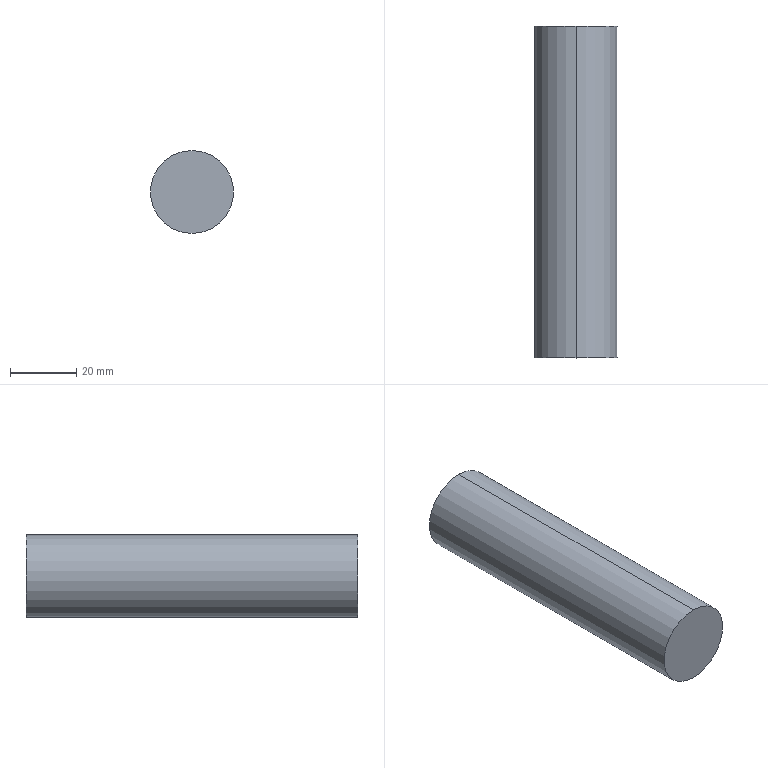Part | SolidWorks | features Extrusion 1 | 1 solid | 4 faces | box 25 x 100 x 25 mm | volume 49087 mm3 | cylinder 2 | plane 2 | commonest cylinder face diameters 25 x2
STEP:
#1=CARTESIAN_POINT('',(0.,100.,12.5));
#2=VERTEX_POINT('',#1);
#3=CARTESIAN_POINT('',(0.,100.,-12.5));
#4=VERTEX_POINT('',#3);
#5=CARTESIAN_POINT('',(0.,100.,0.));
#6=DIRECTION('',(0.,1.,0.));
#7=DIRECTION('',(0.,0.,1.));
#8=AXIS2_PLACEMENT_3D('',#5,#6,#7);
#9=CIRCLE('',#8,12.5);
#10=EDGE_CURVE('',#2,#4,#9,.T.);
#11=ORIENTED_EDGE('',*,*,#10,.F.);
#12=CARTESIAN_POINT('',(0.,0.,12.5));
#13=VERTEX_POINT('',#12);
#14=CARTESIAN_POINT('',(0.,100.,12.5));
#15=DIRECTION('',(0.,-1.,0.));
#16=VECTOR('',#15,1000.);
#17=LINE('',#14,#16);
#18=EDGE_CURVE('',#2,#13,#17,.T.);
#19=ORIENTED_EDGE('',*,*,#18,.T.);
#20=CARTESIAN_POINT('',(0.,0.,-12.5));
#21=VERTEX_POINT('',#20);
#22=CARTESIAN_POINT('',(0.,0.,0.));
#23=DIRECTION('',(0.,1.,0.));
#24=DIRECTION('',(0.,0.,1.));
#25=AXIS2_PLACEMENT_3D('',#22,#23,#24);
#26=CIRCLE('',#25,12.5);
#27=EDGE_CURVE('',#13,#21,#26,.T.);
#28=ORIENTED_EDGE('',*,*,#27,.T.);
#29=CARTESIAN_POINT('',(0.,100.,-12.5));
#30=DIRECTION('',(0.,-1.,0.));
#31=VECTOR('',#30,1000.);
#32=LINE('',#29,#31);
#33=EDGE_CURVE('',#4,#21,#32,.T.);
#34=ORIENTED_EDGE('',*,*,#33,.F.);
#35=EDGE_LOOP('',(#11,#19,#28,#34));
#36=FACE_OUTER_BOUND('',#35,.T.);
#37=CARTESIAN_POINT('',(0.,100.,0.));
#38=DIRECTION('',(0.,-1.,0.));
#39=DIRECTION('',(0.,0.,-1.));
#40=AXIS2_PLACEMENT_3D('',#37,#38,#39);
#41=CYLINDRICAL_SURFACE('',#40,12.5);
#42=ADVANCED_FACE('',(#36),#41,.T.);
#43=ORIENTED_EDGE('',*,*,#18,.F.);
#44=CARTESIAN_POINT('',(0.,100.,0.));
#45=DIRECTION('',(0.,1.,0.));
#46=DIRECTION('',(0.,0.,1.));
#47=AXIS2_PLACEMENT_3D('',#44,#45,#46);
#48=CIRCLE('',#47,12.5);
#49=EDGE_CURVE('',#4,#2,#48,.T.);
#50=ORIENTED_EDGE('',*,*,#49,.F.);
#51=ORIENTED_EDGE('',*,*,#33,.T.);
#52=CARTESIAN_POINT('',(0.,0.,0.));
#53=DIRECTION('',(0.,1.,0.));
#54=DIRECTION('',(0.,0.,1.));
#55=AXIS2_PLACEMENT_3D('',#52,#53,#54);
#56=CIRCLE('',#55,12.5);
#57=EDGE_CURVE('',#21,#13,#56,.T.);
#58=ORIENTED_EDGE('',*,*,#57,.T.);
#59=EDGE_LOOP('',(#43,#50,#51,#58));
#60=FACE_OUTER_BOUND('',#59,.T.);
#61=CARTESIAN_POINT('',(0.,100.,0.));
#62=DIRECTION('',(0.,-1.,0.));
#63=DIRECTION('',(0.,0.,-1.));
#64=AXIS2_PLACEMENT_3D('',#61,#62,#63);
#65=CYLINDRICAL_SURFACE('',#64,12.5);
#66=ADVANCED_FACE('',(#60),#65,.T.);
#67=ORIENTED_EDGE('',*,*,#49,.T.);
#68=ORIENTED_EDGE('',*,*,#10,.T.);
#69=EDGE_LOOP('',(#67,#68));
#70=FACE_OUTER_BOUND('',#69,.T.);
#71=CARTESIAN_POINT('',(0.,100.,0.));
#72=DIRECTION('',(0.,1.,0.));
#73=DIRECTION('',(0.,0.,1.));
#74=AXIS2_PLACEMENT_3D('',#71,#72,#73);
#75=PLANE('',#74);
#76=ADVANCED_FACE('',(#70),#75,.T.);
#77=ORIENTED_EDGE('',*,*,#57,.F.);
#78=ORIENTED_EDGE('',*,*,#27,.F.);
#79=EDGE_LOOP('',(#77,#78));
#80=FACE_OUTER_BOUND('',#79,.T.);
#81=CARTESIAN_POINT('',(0.,0.,0.));
#82=DIRECTION('',(0.,1.,0.));
#83=DIRECTION('',(0.,0.,1.));
#84=AXIS2_PLACEMENT_3D('',#81,#82,#83);
#85=PLANE('',#84);
#86=ADVANCED_FACE('',(#80),#85,.F.);
#87=CLOSED_SHELL('',(#42,#66,#76,#86));
#88=MANIFOLD_SOLID_BREP('',#87);
#89=CARTESIAN_POINT('',(0.,0.,0.));
#90=DIRECTION('',(0.,0.,1.));
#91=DIRECTION('',(1.,0.,0.));
#92=AXIS2_PLACEMENT_3D('',#89,#90,#91);
#93=(LENGTH_UNIT()NAMED_UNIT(*)SI_UNIT(.MILLI.,.METRE.));
#94=UNCERTAINTY_MEASURE_WITH_UNIT(LENGTH_MEASURE(0.00001),#93,'','');
#95=(NAMED_UNIT(*)PLANE_ANGLE_UNIT()SI_UNIT($,.RADIAN.));
#96=(NAMED_UNIT(*)SI_UNIT($,.STERADIAN.)SOLID_ANGLE_UNIT());
#97=(GEOMETRIC_REPRESENTATION_CONTEXT(3)GLOBAL_UNCERTAINTY_ASSIGNED_CONTEXT((#94))GLOBAL_UNIT_ASSIGNED_CONTEXT((#93,#95,#96))REPRESENTATION_CONTEXT('',''));
#98=ADVANCED_BREP_SHAPE_REPRESENTATION('',(#88,#92),#97);